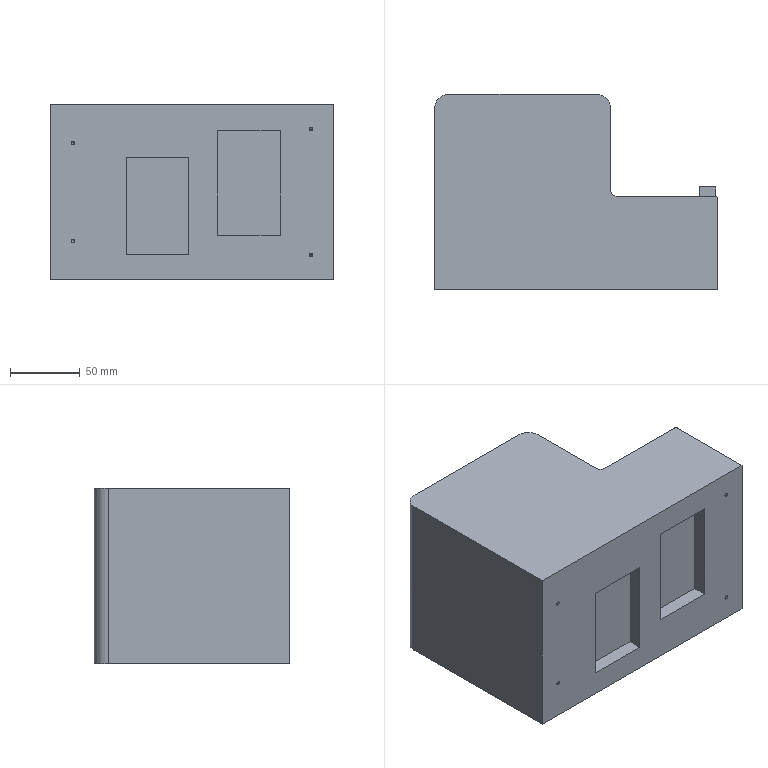Part | 1 solid | 53 faces | box 202.5 x 140 x 126 mm | volume 2802500 mm3 | plane 31 | cylinder 14 | cone 8 | commonest cylinder face diameters 2.5 x8 3 x3 20 x2 8 x1
STEP:
#1=CARTESIAN_POINT('',(16.,11.5,36.25));
#2=VERTEX_POINT('',#1);
#3=CARTESIAN_POINT('',(16.,11.5,33.75));
#4=VERTEX_POINT('',#3);
#5=CARTESIAN_POINT('',(16.,11.5,35.));
#6=DIRECTION('',(0.,-1.,0.));
#7=DIRECTION('',(0.,0.,-1.));
#8=AXIS2_PLACEMENT_3D('',#5,#6,#7);
#9=CIRCLE('',#8,1.25);
#10=EDGE_CURVE('',#2,#4,#9,.T.);
#11=ORIENTED_EDGE('',*,*,#10,.F.);
#12=CARTESIAN_POINT('',(16.,0.,36.25));
#13=VERTEX_POINT('',#12);
#14=CARTESIAN_POINT('',(16.,0.,36.25));
#15=DIRECTION('',(0.,-1.,0.));
#16=VECTOR('',#15,1000.);
#17=LINE('',#14,#16);
#18=EDGE_CURVE('',#2,#13,#17,.T.);
#19=ORIENTED_EDGE('',*,*,#18,.T.);
#20=CARTESIAN_POINT('',(16.,0.,33.75));
#21=VERTEX_POINT('',#20);
#22=CARTESIAN_POINT('',(16.,0.,35.));
#23=DIRECTION('',(0.,-1.,0.));
#24=DIRECTION('',(0.,0.,-1.));
#25=AXIS2_PLACEMENT_3D('',#22,#23,#24);
#26=CIRCLE('',#25,1.25);
#27=EDGE_CURVE('',#13,#21,#26,.T.);
#28=ORIENTED_EDGE('',*,*,#27,.T.);
#29=CARTESIAN_POINT('',(16.,0.,33.75));
#30=DIRECTION('',(0.,-1.,0.));
#31=VECTOR('',#30,1000.);
#32=LINE('',#29,#31);
#33=EDGE_CURVE('',#4,#21,#32,.T.);
#34=ORIENTED_EDGE('',*,*,#33,.F.);
#35=EDGE_LOOP('',(#11,#19,#28,#34));
#36=FACE_OUTER_BOUND('',#35,.T.);
#37=CARTESIAN_POINT('',(16.,0.,35.));
#38=DIRECTION('',(0.,-1.,0.));
#39=DIRECTION('',(0.,0.,-1.));
#40=AXIS2_PLACEMENT_3D('',#37,#38,#39);
#41=CYLINDRICAL_SURFACE('',#40,1.25);
#42=ADVANCED_FACE('',(#36),#41,.F.);
#43=CARTESIAN_POINT('',(16.,12.251,35.));
#44=VERTEX_POINT('',#43);
#45=CARTESIAN_POINT('',(16.,11.5,33.75));
#46=DIRECTION('',(0.,-0.515,-0.8572));
#47=VECTOR('',#46,1000.);
#48=LINE('',#45,#47);
#49=EDGE_CURVE('',#44,#4,#48,.T.);
#50=ORIENTED_EDGE('',*,*,#49,.F.);
#51=CARTESIAN_POINT('',(16.,11.5,36.25));
#52=DIRECTION('',(0.,-0.515,0.8572));
#53=VECTOR('',#52,1000.);
#54=LINE('',#51,#53);
#55=EDGE_CURVE('',#44,#2,#54,.T.);
#56=ORIENTED_EDGE('',*,*,#55,.T.);
#57=ORIENTED_EDGE('',*,*,#10,.T.);
#58=EDGE_LOOP('',(#50,#56,#57));
#59=FACE_OUTER_BOUND('',#58,.T.);
#60=CARTESIAN_POINT('',(16.,11.5,35.));
#61=DIRECTION('',(0.,-1.,0.));
#62=DIRECTION('',(0.,0.,-1.));
#63=AXIS2_PLACEMENT_3D('',#60,#61,#62);
#64=CONICAL_SURFACE('',#63,1.25,1.03);
#65=ADVANCED_FACE('',(#59),#64,.F.);
#66=CARTESIAN_POINT('',(16.,11.5,-33.75));
#67=VERTEX_POINT('',#66);
#68=CARTESIAN_POINT('',(16.,11.5,-36.25));
#69=VERTEX_POINT('',#68);
#70=CARTESIAN_POINT('',(16.,11.5,-35.));
#71=DIRECTION('',(0.,-1.,0.));
#72=DIRECTION('',(0.,0.,-1.));
#73=AXIS2_PLACEMENT_3D('',#70,#71,#72);
#74=CIRCLE('',#73,1.25);
#75=EDGE_CURVE('',#67,#69,#74,.T.);
#76=ORIENTED_EDGE('',*,*,#75,.F.);
#77=CARTESIAN_POINT('',(16.,0.,-33.75));
#78=VERTEX_POINT('',#77);
#79=CARTESIAN_POINT('',(16.,0.,-33.75));
#80=DIRECTION('',(0.,-1.,0.));
#81=VECTOR('',#80,1000.);
#82=LINE('',#79,#81);
#83=EDGE_CURVE('',#67,#78,#82,.T.);
#84=ORIENTED_EDGE('',*,*,#83,.T.);
#85=CARTESIAN_POINT('',(16.,0.,-36.25));
#86=VERTEX_POINT('',#85);
#87=CARTESIAN_POINT('',(16.,0.,-35.));
#88=DIRECTION('',(0.,-1.,0.));
#89=DIRECTION('',(0.,0.,-1.));
#90=AXIS2_PLACEMENT_3D('',#87,#88,#89);
#91=CIRCLE('',#90,1.25);
#92=EDGE_CURVE('',#78,#86,#91,.T.);
#93=ORIENTED_EDGE('',*,*,#92,.T.);
#94=CARTESIAN_POINT('',(16.,0.,-36.25));
#95=DIRECTION('',(0.,-1.,0.));
#96=VECTOR('',#95,1000.);
#97=LINE('',#94,#96);
#98=EDGE_CURVE('',#69,#86,#97,.T.);
#99=ORIENTED_EDGE('',*,*,#98,.F.);
#100=EDGE_LOOP('',(#76,#84,#93,#99));
#101=FACE_OUTER_BOUND('',#100,.T.);
#102=CARTESIAN_POINT('',(16.,0.,-35.));
#103=DIRECTION('',(0.,-1.,0.));
#104=DIRECTION('',(0.,0.,-1.));
#105=AXIS2_PLACEMENT_3D('',#102,#103,#104);
#106=CYLINDRICAL_SURFACE('',#105,1.25);
#107=ADVANCED_FACE('',(#101),#106,.F.);
#108=CARTESIAN_POINT('',(16.,12.251,-35.));
#109=VERTEX_POINT('',#108);
#110=CARTESIAN_POINT('',(16.,11.5,-36.25));
#111=DIRECTION('',(0.,-0.515,-0.8572));
#112=VECTOR('',#111,1000.);
#113=LINE('',#110,#112);
#114=EDGE_CURVE('',#109,#69,#113,.T.);
#115=ORIENTED_EDGE('',*,*,#114,.F.);
#116=CARTESIAN_POINT('',(16.,11.5,-33.75));
#117=DIRECTION('',(0.,-0.515,0.8572));
#118=VECTOR('',#117,1000.);
#119=LINE('',#116,#118);
#120=EDGE_CURVE('',#109,#67,#119,.T.);
#121=ORIENTED_EDGE('',*,*,#120,.T.);
#122=ORIENTED_EDGE('',*,*,#75,.T.);
#123=EDGE_LOOP('',(#115,#121,#122));
#124=FACE_OUTER_BOUND('',#123,.T.);
#125=CARTESIAN_POINT('',(16.,11.5,-35.));
#126=DIRECTION('',(0.,-1.,0.));
#127=DIRECTION('',(0.,0.,-1.));
#128=AXIS2_PLACEMENT_3D('',#125,#126,#127);
#129=CONICAL_SURFACE('',#128,1.25,1.03);
#130=ADVANCED_FACE('',(#124),#129,.F.);
#131=CARTESIAN_POINT('',(186.5,11.5,46.25));
#132=VERTEX_POINT('',#131);
#133=CARTESIAN_POINT('',(186.5,11.5,43.75));
#134=VERTEX_POINT('',#133);
#135=CARTESIAN_POINT('',(186.5,11.5,45.));
#136=DIRECTION('',(0.,-1.,0.));
#137=DIRECTION('',(0.,0.,-1.));
#138=AXIS2_PLACEMENT_3D('',#135,#136,#137);
#139=CIRCLE('',#138,1.25);
#140=EDGE_CURVE('',#132,#134,#139,.T.);
#141=ORIENTED_EDGE('',*,*,#140,.F.);
#142=CARTESIAN_POINT('',(186.5,0.,46.25));
#143=VERTEX_POINT('',#142);
#144=CARTESIAN_POINT('',(186.5,0.,46.25));
#145=DIRECTION('',(0.,-1.,0.));
#146=VECTOR('',#145,1000.);
#147=LINE('',#144,#146);
#148=EDGE_CURVE('',#132,#143,#147,.T.);
#149=ORIENTED_EDGE('',*,*,#148,.T.);
#150=CARTESIAN_POINT('',(186.5,0.,43.75));
#151=VERTEX_POINT('',#150);
#152=CARTESIAN_POINT('',(186.5,0.,45.));
#153=DIRECTION('',(0.,-1.,0.));
#154=DIRECTION('',(0.,0.,-1.));
#155=AXIS2_PLACEMENT_3D('',#152,#153,#154);
#156=CIRCLE('',#155,1.25);
#157=EDGE_CURVE('',#143,#151,#156,.T.);
#158=ORIENTED_EDGE('',*,*,#157,.T.);
#159=CARTESIAN_POINT('',(186.5,0.,43.75));
#160=DIRECTION('',(0.,-1.,0.));
#161=VECTOR('',#160,1000.);
#162=LINE('',#159,#161);
#163=EDGE_CURVE('',#134,#151,#162,.T.);
#164=ORIENTED_EDGE('',*,*,#163,.F.);
#165=EDGE_LOOP('',(#141,#149,#158,#164));
#166=FACE_OUTER_BOUND('',#165,.T.);
#167=CARTESIAN_POINT('',(186.5,0.,45.));
#168=DIRECTION('',(0.,-1.,0.));
#169=DIRECTION('',(0.,0.,-1.));
#170=AXIS2_PLACEMENT_3D('',#167,#168,#169);
#171=CYLINDRICAL_SURFACE('',#170,1.25);
#172=ADVANCED_FACE('',(#166),#171,.F.);
#173=CARTESIAN_POINT('',(186.5,12.251,45.));
#174=VERTEX_POINT('',#173);
#175=CARTESIAN_POINT('',(186.5,11.5,43.75));
#176=DIRECTION('',(0.,-0.515,-0.8572));
#177=VECTOR('',#176,1000.);
#178=LINE('',#175,#177);
#179=EDGE_CURVE('',#174,#134,#178,.T.);
#180=ORIENTED_EDGE('',*,*,#179,.F.);
#181=CARTESIAN_POINT('',(186.5,11.5,46.25));
#182=DIRECTION('',(0.,-0.515,0.8572));
#183=VECTOR('',#182,1000.);
#184=LINE('',#181,#183);
#185=EDGE_CURVE('',#174,#132,#184,.T.);
#186=ORIENTED_EDGE('',*,*,#185,.T.);
#187=ORIENTED_EDGE('',*,*,#140,.T.);
#188=EDGE_LOOP('',(#180,#186,#187));
#189=FACE_OUTER_BOUND('',#188,.T.);
#190=CARTESIAN_POINT('',(186.5,11.5,45.));
#191=DIRECTION('',(0.,-1.,0.));
#192=DIRECTION('',(0.,0.,-1.));
#193=AXIS2_PLACEMENT_3D('',#190,#191,#192);
#194=CONICAL_SURFACE('',#193,1.25,1.03);
#195=ADVANCED_FACE('',(#189),#194,.F.);
#196=CARTESIAN_POINT('',(186.5,11.5,-43.75));
#197=VERTEX_POINT('',#196);
#198=CARTESIAN_POINT('',(186.5,11.5,-46.25));
#199=VERTEX_POINT('',#198);
#200=CARTESIAN_POINT('',(186.5,11.5,-45.));
#201=DIRECTION('',(0.,-1.,0.));
#202=DIRECTION('',(0.,0.,-1.));
#203=AXIS2_PLACEMENT_3D('',#200,#201,#202);
#204=CIRCLE('',#203,1.25);
#205=EDGE_CURVE('',#197,#199,#204,.T.);
#206=ORIENTED_EDGE('',*,*,#205,.F.);
#207=CARTESIAN_POINT('',(186.5,0.,-43.75));
#208=VERTEX_POINT('',#207);
#209=CARTESIAN_POINT('',(186.5,0.,-43.75));
#210=DIRECTION('',(0.,-1.,0.));
#211=VECTOR('',#210,1000.);
#212=LINE('',#209,#211);
#213=EDGE_CURVE('',#197,#208,#212,.T.);
#214=ORIENTED_EDGE('',*,*,#213,.T.);
#215=CARTESIAN_POINT('',(186.5,0.,-46.25));
#216=VERTEX_POINT('',#215);
#217=CARTESIAN_POINT('',(186.5,0.,-45.));
#218=DIRECTION('',(0.,-1.,0.));
#219=DIRECTION('',(0.,0.,-1.));
#220=AXIS2_PLACEMENT_3D('',#217,#218,#219);
#221=CIRCLE('',#220,1.25);
#222=EDGE_CURVE('',#208,#216,#221,.T.);
#223=ORIENTED_EDGE('',*,*,#222,.T.);
#224=CARTESIAN_POINT('',(186.5,0.,-46.25));
#225=DIRECTION('',(0.,-1.,0.));
#226=VECTOR('',#225,1000.);
#227=LINE('',#224,#226);
#228=EDGE_CURVE('',#199,#216,#227,.T.);
#229=ORIENTED_EDGE('',*,*,#228,.F.);
#230=EDGE_LOOP('',(#206,#214,#223,#229));
#231=FACE_OUTER_BOUND('',#230,.T.);
#232=CARTESIAN_POINT('',(186.5,0.,-45.));
#233=DIRECTION('',(0.,-1.,0.));
#234=DIRECTION('',(0.,0.,-1.));
#235=AXIS2_PLACEMENT_3D('',#232,#233,#234);
#236=CYLINDRICAL_SURFACE('',#235,1.25);
#237=ADVANCED_FACE('',(#231),#236,.F.);
#238=CARTESIAN_POINT('',(186.5,12.251,-45.));
#239=VERTEX_POINT('',#238);
#240=CARTESIAN_POINT('',(186.5,11.5,-46.25));
#241=DIRECTION('',(0.,-0.515,-0.8572));
#242=VECTOR('',#241,1000.);
#243=LINE('',#240,#242);
#244=EDGE_CURVE('',#239,#199,#243,.T.);
#245=ORIENTED_EDGE('',*,*,#244,.F.);
#246=CARTESIAN_POINT('',(186.5,11.5,-43.75));
#247=DIRECTION('',(0.,-0.515,0.8572));
#248=VECTOR('',#247,1000.);
#249=LINE('',#246,#248);
#250=EDGE_CURVE('',#239,#197,#249,.T.);
#251=ORIENTED_EDGE('',*,*,#250,.T.);
#252=ORIENTED_EDGE('',*,*,#205,.T.);
#253=EDGE_LOOP('',(#245,#251,#252));
#254=FACE_OUTER_BOUND('',#253,.T.);
#255=CARTESIAN_POINT('',(186.5,11.5,-45.));
#256=DIRECTION('',(0.,-1.,0.));
#257=DIRECTION('',(0.,0.,-1.));
#258=AXIS2_PLACEMENT_3D('',#255,#256,#257);
#259=CONICAL_SURFACE('',#258,1.25,1.03);
#260=ADVANCED_FACE('',(#254),#259,.F.);
#261=CARTESIAN_POINT('',(195.72,57.,-0.5));
#262=VERTEX_POINT('',#261);
#263=CARTESIAN_POINT('',(192.72,57.,-0.5));
#264=VERTEX_POINT('',#263);
#265=CARTESIAN_POINT('',(194.22,57.,-0.5));
#266=DIRECTION('',(0.,1.,0.));
#267=DIRECTION('',(-1.,0.,0.));
#268=AXIS2_PLACEMENT_3D('',#265,#266,#267);
#269=CIRCLE('',#268,1.5);
#270=EDGE_CURVE('',#262,#264,#269,.T.);
#271=ORIENTED_EDGE('',*,*,#270,.F.);
#272=CARTESIAN_POINT('',(195.72,67.,-0.5));
#273=VERTEX_POINT('',#272);
#274=CARTESIAN_POINT('',(195.72,57.,-0.5));
#275=DIRECTION('',(0.,1.,0.));
#276=VECTOR('',#275,1000.);
#277=LINE('',#274,#276);
#278=EDGE_CURVE('',#262,#273,#277,.T.);
#279=ORIENTED_EDGE('',*,*,#278,.T.);
#280=CARTESIAN_POINT('',(192.72,67.,-0.5));
#281=VERTEX_POINT('',#280);
#282=CARTESIAN_POINT('',(194.22,67.,-0.5));
#283=DIRECTION('',(0.,1.,0.));
#284=DIRECTION('',(-1.,0.,0.));
#285=AXIS2_PLACEMENT_3D('',#282,#283,#284);
#286=CIRCLE('',#285,1.5);
#287=EDGE_CURVE('',#273,#281,#286,.T.);
#288=ORIENTED_EDGE('',*,*,#287,.T.);
#289=CARTESIAN_POINT('',(192.72,57.,-0.5));
#290=DIRECTION('',(0.,1.,0.));
#291=VECTOR('',#290,1000.);
#292=LINE('',#289,#291);
#293=EDGE_CURVE('',#264,#281,#292,.T.);
#294=ORIENTED_EDGE('',*,*,#293,.F.);
#295=EDGE_LOOP('',(#271,#279,#288,#294));
#296=FACE_OUTER_BOUND('',#295,.T.);
#297=CARTESIAN_POINT('',(194.22,57.,-0.5));
#298=DIRECTION('',(0.,1.,0.));
#299=DIRECTION('',(-1.,0.,0.));
#300=AXIS2_PLACEMENT_3D('',#297,#298,#299);
#301=CYLINDRICAL_SURFACE('',#300,1.5);
#302=ADVANCED_FACE('',(#296),#301,.F.);
#303=CARTESIAN_POINT('',(194.22,67.,-0.5));
#304=DIRECTION('',(0.,1.,0.));
#305=DIRECTION('',(-1.,0.,0.));
#306=AXIS2_PLACEMENT_3D('',#303,#304,#305);
#307=CIRCLE('',#306,1.5);
#308=EDGE_CURVE('',#281,#273,#307,.T.);
#309=ORIENTED_EDGE('',*,*,#308,.F.);
#310=ORIENTED_EDGE('',*,*,#287,.F.);
#311=EDGE_LOOP('',(#309,#310));
#312=FACE_BOUND('',#311,.T.);
#313=CARTESIAN_POINT('',(201.,67.,-63.));
#314=VERTEX_POINT('',#313);
#315=CARTESIAN_POINT('',(130.,67.,-63.));
#316=VERTEX_POINT('',#315);
#317=CARTESIAN_POINT('',(202.5,67.,-63.));
#318=DIRECTION('',(-1.,0.,0.));
#319=VECTOR('',#318,1000.);
#320=LINE('',#317,#319);
#321=EDGE_CURVE('',#314,#316,#320,.T.);
#322=ORIENTED_EDGE('',*,*,#321,.T.);
#323=CARTESIAN_POINT('',(130.,67.,63.));
#324=VERTEX_POINT('',#323);
#325=CARTESIAN_POINT('',(130.,67.,63.));
#326=DIRECTION('',(0.,0.,1.));
#327=VECTOR('',#326,1000.);
#328=LINE('',#325,#327);
#329=EDGE_CURVE('',#316,#324,#328,.T.);
#330=ORIENTED_EDGE('',*,*,#329,.T.);
#331=CARTESIAN_POINT('',(201.,67.,63.));
#332=VERTEX_POINT('',#331);
#333=CARTESIAN_POINT('',(202.5,67.,63.));
#334=DIRECTION('',(-1.,0.,0.));
#335=VECTOR('',#334,1000.);
#336=LINE('',#333,#335);
#337=EDGE_CURVE('',#332,#324,#336,.T.);
#338=ORIENTED_EDGE('',*,*,#337,.F.);
#339=CARTESIAN_POINT('',(201.,67.,53.5));
#340=VERTEX_POINT('',#339);
#341=CARTESIAN_POINT('',(201.,67.,63.));
#342=DIRECTION('',(0.,0.,-1.));
#343=VECTOR('',#342,1000.);
#344=LINE('',#341,#343);
#345=EDGE_CURVE('',#332,#340,#344,.T.);
#346=ORIENTED_EDGE('',*,*,#345,.T.);
#347=CARTESIAN_POINT('',(190.,67.,53.5));
#348=VERTEX_POINT('',#347);
#349=CARTESIAN_POINT('',(190.,67.,53.5));
#350=DIRECTION('',(1.,0.,0.));
#351=VECTOR('',#350,1000.);
#352=LINE('',#349,#351);
#353=EDGE_CURVE('',#348,#340,#352,.T.);
#354=ORIENTED_EDGE('',*,*,#353,.F.);
#355=CARTESIAN_POINT('',(190.,67.,22.5));
#356=VERTEX_POINT('',#355);
#357=CARTESIAN_POINT('',(190.,67.,22.5));
#358=DIRECTION('',(0.,0.,1.));
#359=VECTOR('',#358,1000.);
#360=LINE('',#357,#359);
#361=EDGE_CURVE('',#356,#348,#360,.T.);
#362=ORIENTED_EDGE('',*,*,#361,.F.);
#363=CARTESIAN_POINT('',(201.,67.,22.5));
#364=VERTEX_POINT('',#363);
#365=CARTESIAN_POINT('',(190.,67.,22.5));
#366=DIRECTION('',(-1.,0.,0.));
#367=VECTOR('',#366,1000.);
#368=LINE('',#365,#367);
#369=EDGE_CURVE('',#364,#356,#368,.T.);
#370=ORIENTED_EDGE('',*,*,#369,.F.);
#371=CARTESIAN_POINT('',(201.,67.,-15.5));
#372=VERTEX_POINT('',#371);
#373=CARTESIAN_POINT('',(201.,67.,63.));
#374=DIRECTION('',(0.,0.,-1.));
#375=VECTOR('',#374,1000.);
#376=LINE('',#373,#375);
#377=EDGE_CURVE('',#364,#372,#376,.T.);
#378=ORIENTED_EDGE('',*,*,#377,.T.);
#379=CARTESIAN_POINT('',(190.,67.,-15.5));
#380=VERTEX_POINT('',#379);
#381=CARTESIAN_POINT('',(190.,67.,-15.5));
#382=DIRECTION('',(1.,0.,0.));
#383=VECTOR('',#382,1000.);
#384=LINE('',#381,#383);
#385=EDGE_CURVE('',#380,#372,#384,.T.);
#386=ORIENTED_EDGE('',*,*,#385,.F.);
#387=CARTESIAN_POINT('',(190.,67.,-46.5));
#388=VERTEX_POINT('',#387);
#389=CARTESIAN_POINT('',(190.,67.,-46.5));
#390=DIRECTION('',(0.,0.,1.));
#391=VECTOR('',#390,1000.);
#392=LINE('',#389,#391);
#393=EDGE_CURVE('',#388,#380,#392,.T.);
#394=ORIENTED_EDGE('',*,*,#393,.F.);
#395=CARTESIAN_POINT('',(201.,67.,-46.5));
#396=VERTEX_POINT('',#395);
#397=CARTESIAN_POINT('',(190.,67.,-46.5));
#398=DIRECTION('',(-1.,0.,0.));
#399=VECTOR('',#398,1000.);
#400=LINE('',#397,#399);
#401=EDGE_CURVE('',#396,#388,#400,.T.);
#402=ORIENTED_EDGE('',*,*,#401,.F.);
#403=CARTESIAN_POINT('',(201.,67.,63.));
#404=DIRECTION('',(0.,0.,-1.));
#405=VECTOR('',#404,1000.);
#406=LINE('',#403,#405);
#407=EDGE_CURVE('',#396,#314,#406,.T.);
#408=ORIENTED_EDGE('',*,*,#407,.T.);
#409=EDGE_LOOP('',(#322,#330,#338,#346,#354,#362,#370,#378,#386,#394,#402,#408));
#410=FACE_OUTER_BOUND('',#409,.T.);
#411=CARTESIAN_POINT('',(202.5,67.,63.));
#412=DIRECTION('',(0.,-1.,0.));
#413=DIRECTION('',(1.,0.,0.));
#414=AXIS2_PLACEMENT_3D('',#411,#412,#413);
#415=PLANE('',#414);
#416=ADVANCED_FACE('',(#312,#410),#415,.F.);
#417=CARTESIAN_POINT('',(116.,140.,63.));
#418=VERTEX_POINT('',#417);
#419=CARTESIAN_POINT('',(10.,140.,63.));
#420=VERTEX_POINT('',#419);
#421=CARTESIAN_POINT('',(126.,140.,63.));
#422=DIRECTION('',(-1.,0.,0.));
#423=VECTOR('',#422,1000.);
#424=LINE('',#421,#423);
#425=EDGE_CURVE('',#418,#420,#424,.T.);
#426=ORIENTED_EDGE('',*,*,#425,.F.);
#427=CARTESIAN_POINT('',(116.,140.,-63.));
#428=VERTEX_POINT('',#427);
#429=CARTESIAN_POINT('',(116.,140.,63.));
#430=DIRECTION('',(0.,0.,-1.));
#431=VECTOR('',#430,1000.);
#432=LINE('',#429,#431);
#433=EDGE_CURVE('',#418,#428,#432,.T.);
#434=ORIENTED_EDGE('',*,*,#433,.T.);
#435=CARTESIAN_POINT('',(10.,140.,-63.));
#436=VERTEX_POINT('',#435);
#437=CARTESIAN_POINT('',(126.,140.,-63.));
#438=DIRECTION('',(-1.,0.,0.));
#439=VECTOR('',#438,1000.);
#440=LINE('',#437,#439);
#441=EDGE_CURVE('',#428,#436,#440,.T.);
#442=ORIENTED_EDGE('',*,*,#441,.T.);
#443=CARTESIAN_POINT('',(10.,140.,63.));
#444=DIRECTION('',(0.,0.,1.));
#445=VECTOR('',#444,1000.);
#446=LINE('',#443,#445);
#447=EDGE_CURVE('',#436,#420,#446,.T.);
#448=ORIENTED_EDGE('',*,*,#447,.T.);
#449=EDGE_LOOP('',(#426,#434,#442,#448));
#450=FACE_OUTER_BOUND('',#449,.T.);
#451=CARTESIAN_POINT('',(126.,140.,63.));
#452=DIRECTION('',(0.,-1.,0.));
#453=DIRECTION('',(1.,0.,0.));
#454=AXIS2_PLACEMENT_3D('',#451,#452,#453);
#455=PLANE('',#454);
#456=ADVANCED_FACE('',(#450),#455,.F.);
#457=CARTESIAN_POINT('',(0.,130.,63.));
#458=VERTEX_POINT('',#457);
#459=CARTESIAN_POINT('',(0.,0.,63.));
#460=VERTEX_POINT('',#459);
#461=CARTESIAN_POINT('',(0.,140.,63.));
#462=DIRECTION('',(0.,-1.,0.));
#463=VECTOR('',#462,1000.);
#464=LINE('',#461,#463);
#465=EDGE_CURVE('',#458,#460,#464,.T.);
#466=ORIENTED_EDGE('',*,*,#465,.F.);
#467=CARTESIAN_POINT('',(0.,130.,-63.));
#468=VERTEX_POINT('',#467);
#469=CARTESIAN_POINT('',(0.,130.,63.));
#470=DIRECTION('',(0.,0.,-1.));
#471=VECTOR('',#470,1000.);
#472=LINE('',#469,#471);
#473=EDGE_CURVE('',#458,#468,#472,.T.);
#474=ORIENTED_EDGE('',*,*,#473,.T.);
#475=CARTESIAN_POINT('',(0.,0.,-63.));
#476=VERTEX_POINT('',#475);
#477=CARTESIAN_POINT('',(0.,140.,-63.));
#478=DIRECTION('',(0.,-1.,0.));
#479=VECTOR('',#478,1000.);
#480=LINE('',#477,#479);
#481=EDGE_CURVE('',#468,#476,#480,.T.);
#482=ORIENTED_EDGE('',*,*,#481,.T.);
#483=CARTESIAN_POINT('',(0.,0.,63.));
#484=DIRECTION('',(0.,0.,-1.));
#485=VECTOR('',#484,1000.);
#486=LINE('',#483,#485);
#487=EDGE_CURVE('',#460,#476,#486,.T.);
#488=ORIENTED_EDGE('',*,*,#487,.F.);
#489=EDGE_LOOP('',(#466,#474,#482,#488));
#490=FACE_OUTER_BOUND('',#489,.T.);
#491=CARTESIAN_POINT('',(0.,140.,63.));
#492=DIRECTION('',(1.,0.,0.));
#493=DIRECTION('',(0.,1.,0.));
#494=AXIS2_PLACEMENT_3D('',#491,#492,#493);
#495=PLANE('',#494);
#496=ADVANCED_FACE('',(#490),#495,.F.);
#497=CARTESIAN_POINT('',(164.5,0.,44.));
#498=VERTEX_POINT('',#497);
#499=CARTESIAN_POINT('',(119.5,0.,44.));
#500=VERTEX_POINT('',#499);
#501=CARTESIAN_POINT('',(119.5,0.,44.));
#502=DIRECTION('',(-1.,0.,0.));
#503=VECTOR('',#502,1000.);
#504=LINE('',#501,#503);
#505=EDGE_CURVE('',#498,#500,#504,.T.);
#506=ORIENTED_EDGE('',*,*,#505,.F.);
#507=CARTESIAN_POINT('',(164.5,0.,-31.));
#508=VERTEX_POINT('',#507);
#509=CARTESIAN_POINT('',(164.5,0.,44.));
#510=DIRECTION('',(0.,0.,1.));
#511=VECTOR('',#510,1000.);
#512=LINE('',#509,#511);
#513=EDGE_CURVE('',#508,#498,#512,.T.);
#514=ORIENTED_EDGE('',*,*,#513,.F.);
#515=CARTESIAN_POINT('',(119.5,0.,-31.));
#516=VERTEX_POINT('',#515);
#517=CARTESIAN_POINT('',(119.5,0.,-31.));
#518=DIRECTION('',(1.,0.,0.));
#519=VECTOR('',#518,1000.);
#520=LINE('',#517,#519);
#521=EDGE_CURVE('',#516,#508,#520,.T.);
#522=ORIENTED_EDGE('',*,*,#521,.F.);
#523=CARTESIAN_POINT('',(119.5,0.,44.));
#524=DIRECTION('',(0.,0.,-1.));
#525=VECTOR('',#524,1000.);
#526=LINE('',#523,#525);
#527=EDGE_CURVE('',#500,#516,#526,.T.);
#528=ORIENTED_EDGE('',*,*,#527,.F.);
#529=EDGE_LOOP('',(#506,#514,#522,#528));
#530=FACE_BOUND('',#529,.T.);
#531=CARTESIAN_POINT('',(99.,0.,25.));
#532=VERTEX_POINT('',#531);
#533=CARTESIAN_POINT('',(54.,0.,25.));
#534=VERTEX_POINT('',#533);
#535=CARTESIAN_POINT('',(54.,0.,25.));
#536=DIRECTION('',(-1.,0.,0.));
#537=VECTOR('',#536,1000.);
#538=LINE('',#535,#537);
#539=EDGE_CURVE('',#532,#534,#538,.T.);
#540=ORIENTED_EDGE('',*,*,#539,.F.);
#541=CARTESIAN_POINT('',(99.,0.,-45.));
#542=VERTEX_POINT('',#541);
#543=CARTESIAN_POINT('',(99.,0.,25.));
#544=DIRECTION('',(0.,0.,1.));
#545=VECTOR('',#544,1000.);
#546=LINE('',#543,#545);
#547=EDGE_CURVE('',#542,#532,#546,.T.);
#548=ORIENTED_EDGE('',*,*,#547,.F.);
#549=CARTESIAN_POINT('',(54.,0.,-45.));
#550=VERTEX_POINT('',#549);
#551=CARTESIAN_POINT('',(54.,0.,-45.));
#552=DIRECTION('',(1.,0.,0.));
#553=VECTOR('',#552,1000.);
#554=LINE('',#551,#553);
#555=EDGE_CURVE('',#550,#542,#554,.T.);
#556=ORIENTED_EDGE('',*,*,#555,.F.);
#557=CARTESIAN_POINT('',(54.,0.,25.));
#558=DIRECTION('',(0.,0.,-1.));
#559=VECTOR('',#558,1000.);
#560=LINE('',#557,#559);
#561=EDGE_CURVE('',#534,#550,#560,.T.);
#562=ORIENTED_EDGE('',*,*,#561,.F.);
#563=EDGE_LOOP('',(#540,#548,#556,#562));
#564=FACE_BOUND('',#563,.T.);
#565=CARTESIAN_POINT('',(16.,0.,35.));
#566=DIRECTION('',(0.,-1.,0.));
#567=DIRECTION('',(0.,0.,-1.));
#568=AXIS2_PLACEMENT_3D('',#565,#566,#567);
#569=CIRCLE('',#568,1.25);
#570=EDGE_CURVE('',#21,#13,#569,.T.);
#571=ORIENTED_EDGE('',*,*,#570,.F.);
#572=ORIENTED_EDGE('',*,*,#27,.F.);
#573=EDGE_LOOP('',(#571,#572));
#574=FACE_BOUND('',#573,.T.);
#575=CARTESIAN_POINT('',(16.,0.,-35.));
#576=DIRECTION('',(0.,-1.,0.));
#577=DIRECTION('',(0.,0.,-1.));
#578=AXIS2_PLACEMENT_3D('',#575,#576,#577);
#579=CIRCLE('',#578,1.25);
#580=EDGE_CURVE('',#86,#78,#579,.T.);
#581=ORIENTED_EDGE('',*,*,#580,.F.);
#582=ORIENTED_EDGE('',*,*,#92,.F.);
#583=EDGE_LOOP('',(#581,#582));
#584=FACE_BOUND('',#583,.T.);
#585=CARTESIAN_POINT('',(186.5,0.,45.));
#586=DIRECTION('',(0.,-1.,0.));
#587=DIRECTION('',(0.,0.,-1.));
#588=AXIS2_PLACEMENT_3D('',#585,#586,#587);
#589=CIRCLE('',#588,1.25);
#590=EDGE_CURVE('',#151,#143,#589,.T.);
#591=ORIENTED_EDGE('',*,*,#590,.F.);
#592=ORIENTED_EDGE('',*,*,#157,.F.);
#593=EDGE_LOOP('',(#591,#592));
#594=FACE_BOUND('',#593,.T.);
#595=CARTESIAN_POINT('',(186.5,0.,-45.));
#596=DIRECTION('',(0.,-1.,0.));
#597=DIRECTION('',(0.,0.,-1.));
#598=AXIS2_PLACEMENT_3D('',#595,#596,#597);
#599=CIRCLE('',#598,1.25);
#600=EDGE_CURVE('',#216,#208,#599,.T.);
#601=ORIENTED_EDGE('',*,*,#600,.F.);
#602=ORIENTED_EDGE('',*,*,#222,.F.);
#603=EDGE_LOOP('',(#601,#602));
#604=FACE_BOUND('',#603,.T.);
#605=CARTESIAN_POINT('',(202.5,0.,-63.));
#606=VERTEX_POINT('',#605);
#607=CARTESIAN_POINT('',(0.,0.,-63.));
#608=DIRECTION('',(1.,0.,0.));
#609=VECTOR('',#608,1000.);
#610=LINE('',#607,#609);
#611=EDGE_CURVE('',#476,#606,#610,.T.);
#612=ORIENTED_EDGE('',*,*,#611,.T.);
#613=CARTESIAN_POINT('',(202.5,0.,63.));
#614=VERTEX_POINT('',#613);
#615=CARTESIAN_POINT('',(202.5,0.,63.));
#616=DIRECTION('',(0.,0.,-1.));
#617=VECTOR('',#616,1000.);
#618=LINE('',#615,#617);
#619=EDGE_CURVE('',#614,#606,#618,.T.);
#620=ORIENTED_EDGE('',*,*,#619,.F.);
#621=CARTESIAN_POINT('',(0.,0.,63.));
#622=DIRECTION('',(1.,0.,0.));
#623=VECTOR('',#622,1000.);
#624=LINE('',#621,#623);
#625=EDGE_CURVE('',#460,#614,#624,.T.);
#626=ORIENTED_EDGE('',*,*,#625,.F.);
#627=ORIENTED_EDGE('',*,*,#487,.T.);
#628=EDGE_LOOP('',(#612,#620,#626,#627));
#629=FACE_OUTER_BOUND('',#628,.T.);
#630=CARTESIAN_POINT('',(0.,0.,63.));
#631=DIRECTION('',(0.,1.,0.));
#632=DIRECTION('',(0.,0.,1.));
#633=AXIS2_PLACEMENT_3D('',#630,#631,#632);
#634=PLANE('',#633);
#635=ADVANCED_FACE('',(#530,#564,#574,#584,#594,#604,#629),#634,.F.);
#636=CARTESIAN_POINT('',(202.5,65.5,-63.));
#637=VERTEX_POINT('',#636);
#638=CARTESIAN_POINT('',(202.5,0.,-63.));
#639=DIRECTION('',(0.,1.,0.));
#640=VECTOR('',#639,1000.);
#641=LINE('',#638,#640);
#642=EDGE_CURVE('',#606,#637,#641,.T.);
#643=ORIENTED_EDGE('',*,*,#642,.T.);
#644=CARTESIAN_POINT('',(202.5,65.5,63.));
#645=VERTEX_POINT('',#644);
#646=CARTESIAN_POINT('',(202.5,65.5,63.));
#647=DIRECTION('',(0.,0.,1.));
#648=VECTOR('',#647,1000.);
#649=LINE('',#646,#648);
#650=EDGE_CURVE('',#637,#645,#649,.T.);
#651=ORIENTED_EDGE('',*,*,#650,.T.);
#652=CARTESIAN_POINT('',(202.5,0.,63.));
#653=DIRECTION('',(0.,1.,0.));
#654=VECTOR('',#653,1000.);
#655=LINE('',#652,#654);
#656=EDGE_CURVE('',#614,#645,#655,.T.);
#657=ORIENTED_EDGE('',*,*,#656,.F.);
#658=ORIENTED_EDGE('',*,*,#619,.T.);
#659=EDGE_LOOP('',(#643,#651,#657,#658));
#660=FACE_OUTER_BOUND('',#659,.T.);
#661=CARTESIAN_POINT('',(202.5,0.,63.));
#662=DIRECTION('',(-1.,0.,0.));
#663=DIRECTION('',(0.,0.,1.));
#664=AXIS2_PLACEMENT_3D('',#661,#662,#663);
#665=PLANE('',#664);
#666=ADVANCED_FACE('',(#660),#665,.F.);
#667=CARTESIAN_POINT('',(126.,71.,63.));
#668=VERTEX_POINT('',#667);
#669=CARTESIAN_POINT('',(126.,130.,63.));
#670=VERTEX_POINT('',#669);
#671=CARTESIAN_POINT('',(126.,67.,63.));
#672=DIRECTION('',(0.,1.,0.));
#673=VECTOR('',#672,1000.);
#674=LINE('',#671,#673);
#675=EDGE_CURVE('',#668,#670,#674,.T.);
#676=ORIENTED_EDGE('',*,*,#675,.F.);
#677=CARTESIAN_POINT('',(126.,71.,-63.));
#678=VERTEX_POINT('',#677);
#679=CARTESIAN_POINT('',(126.,71.,-63.));
#680=DIRECTION('',(0.,0.,-1.));
#681=VECTOR('',#680,1000.);
#682=LINE('',#679,#681);
#683=EDGE_CURVE('',#668,#678,#682,.T.);
#684=ORIENTED_EDGE('',*,*,#683,.T.);
#685=CARTESIAN_POINT('',(126.,130.,-63.));
#686=VERTEX_POINT('',#685);
#687=CARTESIAN_POINT('',(126.,67.,-63.));
#688=DIRECTION('',(0.,1.,0.));
#689=VECTOR('',#688,1000.);
#690=LINE('',#687,#689);
#691=EDGE_CURVE('',#678,#686,#690,.T.);
#692=ORIENTED_EDGE('',*,*,#691,.T.);
#693=CARTESIAN_POINT('',(126.,130.,63.));
#694=DIRECTION('',(0.,0.,1.));
#695=VECTOR('',#694,1000.);
#696=LINE('',#693,#695);
#697=EDGE_CURVE('',#686,#670,#696,.T.);
#698=ORIENTED_EDGE('',*,*,#697,.T.);
#699=EDGE_LOOP('',(#676,#684,#692,#698));
#700=FACE_OUTER_BOUND('',#699,.T.);
#701=CARTESIAN_POINT('',(126.,67.,63.));
#702=DIRECTION('',(-1.,0.,0.));
#703=DIRECTION('',(0.,0.,1.));
#704=AXIS2_PLACEMENT_3D('',#701,#702,#703);
#705=PLANE('',#704);
#706=ADVANCED_FACE('',(#700),#705,.F.);
#707=ORIENTED_EDGE('',*,*,#656,.T.);
#708=CARTESIAN_POINT('',(201.,65.5,63.));
#709=DIRECTION('',(0.,0.,1.));
#710=DIRECTION('',(1.,0.,0.));
#711=AXIS2_PLACEMENT_3D('',#708,#709,#710);
#712=CIRCLE('',#711,1.5);
#713=EDGE_CURVE('',#645,#332,#712,.T.);
#714=ORIENTED_EDGE('',*,*,#713,.T.);
#715=ORIENTED_EDGE('',*,*,#337,.T.);
#716=CARTESIAN_POINT('',(130.,71.,63.));
#717=DIRECTION('',(0.,0.,-1.));
#718=DIRECTION('',(1.,0.,0.));
#719=AXIS2_PLACEMENT_3D('',#716,#717,#718);
#720=CIRCLE('',#719,4.);
#721=EDGE_CURVE('',#324,#668,#720,.T.);
#722=ORIENTED_EDGE('',*,*,#721,.T.);
#723=ORIENTED_EDGE('',*,*,#675,.T.);
#724=CARTESIAN_POINT('',(116.,130.,63.));
#725=DIRECTION('',(0.,0.,1.));
#726=DIRECTION('',(1.,0.,0.));
#727=AXIS2_PLACEMENT_3D('',#724,#725,#726);
#728=CIRCLE('',#727,10.);
#729=EDGE_CURVE('',#670,#418,#728,.T.);
#730=ORIENTED_EDGE('',*,*,#729,.T.);
#731=ORIENTED_EDGE('',*,*,#425,.T.);
#732=CARTESIAN_POINT('',(10.,130.,63.));
#733=DIRECTION('',(0.,0.,1.));
#734=DIRECTION('',(1.,0.,0.));
#735=AXIS2_PLACEMENT_3D('',#732,#733,#734);
#736=CIRCLE('',#735,10.);
#737=EDGE_CURVE('',#420,#458,#736,.T.);
#738=ORIENTED_EDGE('',*,*,#737,.T.);
#739=ORIENTED_EDGE('',*,*,#465,.T.);
#740=ORIENTED_EDGE('',*,*,#625,.T.);
#741=EDGE_LOOP('',(#707,#714,#715,#722,#723,#730,#731,#738,#739,#740));
#742=FACE_OUTER_BOUND('',#741,.T.);
#743=CARTESIAN_POINT('',(0.,0.,63.));
#744=DIRECTION('',(0.,0.,1.));
#745=DIRECTION('',(1.,0.,0.));
#746=AXIS2_PLACEMENT_3D('',#743,#744,#745);
#747=PLANE('',#746);
#748=ADVANCED_FACE('',(#742),#747,.T.);
#749=ORIENTED_EDGE('',*,*,#321,.F.);
#750=CARTESIAN_POINT('',(201.,65.5,-63.));
#751=DIRECTION('',(0.,0.,-1.));
#752=DIRECTION('',(1.,0.,0.));
#753=AXIS2_PLACEMENT_3D('',#750,#751,#752);
#754=CIRCLE('',#753,1.5);
#755=EDGE_CURVE('',#314,#637,#754,.T.);
#756=ORIENTED_EDGE('',*,*,#755,.T.);
#757=ORIENTED_EDGE('',*,*,#642,.F.);
#758=ORIENTED_EDGE('',*,*,#611,.F.);
#759=ORIENTED_EDGE('',*,*,#481,.F.);
#760=CARTESIAN_POINT('',(10.,130.,-63.));
#761=DIRECTION('',(0.,0.,-1.));
#762=DIRECTION('',(1.,0.,0.));
#763=AXIS2_PLACEMENT_3D('',#760,#761,#762);
#764=CIRCLE('',#763,10.);
#765=EDGE_CURVE('',#468,#436,#764,.T.);
#766=ORIENTED_EDGE('',*,*,#765,.T.);
#767=ORIENTED_EDGE('',*,*,#441,.F.);
#768=CARTESIAN_POINT('',(116.,130.,-63.));
#769=DIRECTION('',(0.,0.,-1.));
#770=DIRECTION('',(1.,0.,0.));
#771=AXIS2_PLACEMENT_3D('',#768,#769,#770);
#772=CIRCLE('',#771,10.);
#773=EDGE_CURVE('',#428,#686,#772,.T.);
#774=ORIENTED_EDGE('',*,*,#773,.T.);
#775=ORIENTED_EDGE('',*,*,#691,.F.);
#776=CARTESIAN_POINT('',(130.,71.,-63.));
#777=DIRECTION('',(0.,0.,1.));
#778=DIRECTION('',(1.,0.,0.));
#779=AXIS2_PLACEMENT_3D('',#776,#777,#778);
#780=CIRCLE('',#779,4.);
#781=EDGE_CURVE('',#678,#316,#780,.T.);
#782=ORIENTED_EDGE('',*,*,#781,.T.);
#783=EDGE_LOOP('',(#749,#756,#757,#758,#759,#766,#767,#774,#775,#782));
#784=FACE_OUTER_BOUND('',#783,.T.);
#785=CARTESIAN_POINT('',(0.,0.,-63.));
#786=DIRECTION('',(0.,0.,1.));
#787=DIRECTION('',(1.,0.,0.));
#788=AXIS2_PLACEMENT_3D('',#785,#786,#787);
#789=PLANE('',#788);
#790=ADVANCED_FACE('',(#784),#789,.F.);
#791=ORIENTED_EDGE('',*,*,#729,.F.);
#792=ORIENTED_EDGE('',*,*,#697,.F.);
#793=ORIENTED_EDGE('',*,*,#773,.F.);
#794=ORIENTED_EDGE('',*,*,#433,.F.);
#795=EDGE_LOOP('',(#791,#792,#793,#794));
#796=FACE_OUTER_BOUND('',#795,.T.);
#797=CARTESIAN_POINT('',(116.,130.,63.));
#798=DIRECTION('',(0.,0.,-1.));
#799=DIRECTION('',(-1.,0.,0.));
#800=AXIS2_PLACEMENT_3D('',#797,#798,#799);
#801=CYLINDRICAL_SURFACE('',#800,10.);
#802=ADVANCED_FACE('',(#796),#801,.T.);
#803=ORIENTED_EDGE('',*,*,#737,.F.);
#804=ORIENTED_EDGE('',*,*,#447,.F.);
#805=ORIENTED_EDGE('',*,*,#765,.F.);
#806=ORIENTED_EDGE('',*,*,#473,.F.);
#807=EDGE_LOOP('',(#803,#804,#805,#806));
#808=FACE_OUTER_BOUND('',#807,.T.);
#809=CARTESIAN_POINT('',(10.,130.,63.));
#810=DIRECTION('',(0.,0.,-1.));
#811=DIRECTION('',(-1.,0.,0.));
#812=AXIS2_PLACEMENT_3D('',#809,#810,#811);
#813=CYLINDRICAL_SURFACE('',#812,10.);
#814=ADVANCED_FACE('',(#808),#813,.T.);
#815=ORIENTED_EDGE('',*,*,#713,.F.);
#816=ORIENTED_EDGE('',*,*,#650,.F.);
#817=ORIENTED_EDGE('',*,*,#755,.F.);
#818=ORIENTED_EDGE('',*,*,#407,.F.);
#819=CARTESIAN_POINT('',(201.,67.,63.));
#820=DIRECTION('',(0.,0.,-1.));
#821=VECTOR('',#820,1000.);
#822=LINE('',#819,#821);
#823=EDGE_CURVE('',#372,#396,#822,.T.);
#824=ORIENTED_EDGE('',*,*,#823,.F.);
#825=ORIENTED_EDGE('',*,*,#377,.F.);
#826=CARTESIAN_POINT('',(201.,67.,63.));
#827=DIRECTION('',(0.,0.,-1.));
#828=VECTOR('',#827,1000.);
#829=LINE('',#826,#828);
#830=EDGE_CURVE('',#340,#364,#829,.T.);
#831=ORIENTED_EDGE('',*,*,#830,.F.);
#832=ORIENTED_EDGE('',*,*,#345,.F.);
#833=EDGE_LOOP('',(#815,#816,#817,#818,#824,#825,#831,#832));
#834=FACE_OUTER_BOUND('',#833,.T.);
#835=CARTESIAN_POINT('',(201.,65.5,63.));
#836=DIRECTION('',(0.,0.,-1.));
#837=DIRECTION('',(-1.,0.,0.));
#838=AXIS2_PLACEMENT_3D('',#835,#836,#837);
#839=CYLINDRICAL_SURFACE('',#838,1.5);
#840=ADVANCED_FACE('',(#834),#839,.T.);
#841=ORIENTED_EDGE('',*,*,#278,.F.);
#842=CARTESIAN_POINT('',(194.22,57.,-0.5));
#843=DIRECTION('',(0.,1.,0.));
#844=DIRECTION('',(-1.,0.,0.));
#845=AXIS2_PLACEMENT_3D('',#842,#843,#844);
#846=CIRCLE('',#845,1.5);
#847=EDGE_CURVE('',#264,#262,#846,.T.);
#848=ORIENTED_EDGE('',*,*,#847,.F.);
#849=ORIENTED_EDGE('',*,*,#293,.T.);
#850=ORIENTED_EDGE('',*,*,#308,.T.);
#851=EDGE_LOOP('',(#841,#848,#849,#850));
#852=FACE_OUTER_BOUND('',#851,.T.);
#853=CARTESIAN_POINT('',(194.22,57.,-0.5));
#854=DIRECTION('',(0.,1.,0.));
#855=DIRECTION('',(-1.,0.,0.));
#856=AXIS2_PLACEMENT_3D('',#853,#854,#855);
#857=CYLINDRICAL_SURFACE('',#856,1.5);
#858=ADVANCED_FACE('',(#852),#857,.F.);
#859=ORIENTED_EDGE('',*,*,#847,.T.);
#860=ORIENTED_EDGE('',*,*,#270,.T.);
#861=EDGE_LOOP('',(#859,#860));
#862=FACE_OUTER_BOUND('',#861,.T.);
#863=CARTESIAN_POINT('',(194.22,57.,-0.5));
#864=DIRECTION('',(0.,1.,0.));
#865=DIRECTION('',(-1.,0.,0.));
#866=AXIS2_PLACEMENT_3D('',#863,#864,#865);
#867=PLANE('',#866);
#868=ADVANCED_FACE('',(#862),#867,.T.);
#869=ORIENTED_EDGE('',*,*,#361,.T.);
#870=CARTESIAN_POINT('',(190.,73.5,53.5));
#871=VERTEX_POINT('',#870);
#872=CARTESIAN_POINT('',(190.,73.5,53.5));
#873=DIRECTION('',(0.,-1.,0.));
#874=VECTOR('',#873,1000.);
#875=LINE('',#872,#874);
#876=EDGE_CURVE('',#871,#348,#875,.T.);
#877=ORIENTED_EDGE('',*,*,#876,.F.);
#878=CARTESIAN_POINT('',(190.,73.5,22.5));
#879=VERTEX_POINT('',#878);
#880=CARTESIAN_POINT('',(190.,73.5,22.5));
#881=DIRECTION('',(0.,0.,1.));
#882=VECTOR('',#881,1000.);
#883=LINE('',#880,#882);
#884=EDGE_CURVE('',#879,#871,#883,.T.);
#885=ORIENTED_EDGE('',*,*,#884,.F.);
#886=CARTESIAN_POINT('',(190.,73.5,22.5));
#887=DIRECTION('',(0.,-1.,0.));
#888=VECTOR('',#887,1000.);
#889=LINE('',#886,#888);
#890=EDGE_CURVE('',#879,#356,#889,.T.);
#891=ORIENTED_EDGE('',*,*,#890,.T.);
#892=EDGE_LOOP('',(#869,#877,#885,#891));
#893=FACE_OUTER_BOUND('',#892,.T.);
#894=CARTESIAN_POINT('',(190.,73.5,22.5));
#895=DIRECTION('',(1.,0.,0.));
#896=DIRECTION('',(0.,1.,0.));
#897=AXIS2_PLACEMENT_3D('',#894,#895,#896);
#898=PLANE('',#897);
#899=ADVANCED_FACE('',(#893),#898,.F.);
#900=ORIENTED_EDGE('',*,*,#353,.T.);
#901=CARTESIAN_POINT('',(201.5,67.,53.5));
#902=VERTEX_POINT('',#901);
#903=CARTESIAN_POINT('',(190.,67.,53.5));
#904=DIRECTION('',(1.,0.,0.));
#905=VECTOR('',#904,1000.);
#906=LINE('',#903,#905);
#907=EDGE_CURVE('',#340,#902,#906,.T.);
#908=ORIENTED_EDGE('',*,*,#907,.T.);
#909=CARTESIAN_POINT('',(201.5,73.5,53.5));
#910=VERTEX_POINT('',#909);
#911=CARTESIAN_POINT('',(201.5,73.5,53.5));
#912=DIRECTION('',(0.,-1.,0.));
#913=VECTOR('',#912,1000.);
#914=LINE('',#911,#913);
#915=EDGE_CURVE('',#910,#902,#914,.T.);
#916=ORIENTED_EDGE('',*,*,#915,.F.);
#917=CARTESIAN_POINT('',(190.,73.5,53.5));
#918=DIRECTION('',(1.,0.,0.));
#919=VECTOR('',#918,1000.);
#920=LINE('',#917,#919);
#921=EDGE_CURVE('',#871,#910,#920,.T.);
#922=ORIENTED_EDGE('',*,*,#921,.F.);
#923=ORIENTED_EDGE('',*,*,#876,.T.);
#924=EDGE_LOOP('',(#900,#908,#916,#922,#923));
#925=FACE_OUTER_BOUND('',#924,.T.);
#926=CARTESIAN_POINT('',(190.,73.5,53.5));
#927=DIRECTION('',(0.,0.,-1.));
#928=DIRECTION('',(-1.,0.,0.));
#929=AXIS2_PLACEMENT_3D('',#926,#927,#928);
#930=PLANE('',#929);
#931=ADVANCED_FACE('',(#925),#930,.F.);
#932=CARTESIAN_POINT('',(201.5,67.,22.5));
#933=VERTEX_POINT('',#932);
#934=CARTESIAN_POINT('',(201.5,67.,22.5));
#935=DIRECTION('',(0.,0.,-1.));
#936=VECTOR('',#935,1000.);
#937=LINE('',#934,#936);
#938=EDGE_CURVE('',#902,#933,#937,.T.);
#939=ORIENTED_EDGE('',*,*,#938,.T.);
#940=CARTESIAN_POINT('',(201.5,73.5,22.5));
#941=VERTEX_POINT('',#940);
#942=CARTESIAN_POINT('',(201.5,73.5,22.5));
#943=DIRECTION('',(0.,-1.,0.));
#944=VECTOR('',#943,1000.);
#945=LINE('',#942,#944);
#946=EDGE_CURVE('',#941,#933,#945,.T.);
#947=ORIENTED_EDGE('',*,*,#946,.F.);
#948=CARTESIAN_POINT('',(201.5,73.5,22.5));
#949=DIRECTION('',(0.,0.,-1.));
#950=VECTOR('',#949,1000.);
#951=LINE('',#948,#950);
#952=EDGE_CURVE('',#910,#941,#951,.T.);
#953=ORIENTED_EDGE('',*,*,#952,.F.);
#954=ORIENTED_EDGE('',*,*,#915,.T.);
#955=EDGE_LOOP('',(#939,#947,#953,#954));
#956=FACE_OUTER_BOUND('',#955,.T.);
#957=CARTESIAN_POINT('',(201.5,73.5,22.5));
#958=DIRECTION('',(-1.,0.,0.));
#959=DIRECTION('',(0.,-1.,0.));
#960=AXIS2_PLACEMENT_3D('',#957,#958,#959);
#961=PLANE('',#960);
#962=ADVANCED_FACE('',(#956),#961,.F.);
#963=CARTESIAN_POINT('',(190.,67.,22.5));
#964=DIRECTION('',(-1.,0.,0.));
#965=VECTOR('',#964,1000.);
#966=LINE('',#963,#965);
#967=EDGE_CURVE('',#933,#364,#966,.T.);
#968=ORIENTED_EDGE('',*,*,#967,.T.);
#969=ORIENTED_EDGE('',*,*,#369,.T.);
#970=ORIENTED_EDGE('',*,*,#890,.F.);
#971=CARTESIAN_POINT('',(190.,73.5,22.5));
#972=DIRECTION('',(-1.,0.,0.));
#973=VECTOR('',#972,1000.);
#974=LINE('',#971,#973);
#975=EDGE_CURVE('',#941,#879,#974,.T.);
#976=ORIENTED_EDGE('',*,*,#975,.F.);
#977=ORIENTED_EDGE('',*,*,#946,.T.);
#978=EDGE_LOOP('',(#968,#969,#970,#976,#977));
#979=FACE_OUTER_BOUND('',#978,.T.);
#980=CARTESIAN_POINT('',(190.,73.5,22.5));
#981=DIRECTION('',(0.,0.,1.));
#982=DIRECTION('',(1.,0.,0.));
#983=AXIS2_PLACEMENT_3D('',#980,#981,#982);
#984=PLANE('',#983);
#985=ADVANCED_FACE('',(#979),#984,.F.);
#986=ORIENTED_EDGE('',*,*,#884,.T.);
#987=ORIENTED_EDGE('',*,*,#921,.T.);
#988=ORIENTED_EDGE('',*,*,#952,.T.);
#989=ORIENTED_EDGE('',*,*,#975,.T.);
#990=EDGE_LOOP('',(#986,#987,#988,#989));
#991=FACE_OUTER_BOUND('',#990,.T.);
#992=CARTESIAN_POINT('',(0.,73.5,0.));
#993=DIRECTION('',(0.,1.,0.));
#994=DIRECTION('',(-1.,0.,0.));
#995=AXIS2_PLACEMENT_3D('',#992,#993,#994);
#996=PLANE('',#995);
#997=ADVANCED_FACE('',(#991),#996,.T.);
#998=ORIENTED_EDGE('',*,*,#830,.T.);
#999=ORIENTED_EDGE('',*,*,#967,.F.);
#1000=ORIENTED_EDGE('',*,*,#938,.F.);
#1001=ORIENTED_EDGE('',*,*,#907,.F.);
#1002=EDGE_LOOP('',(#998,#999,#1000,#1001));
#1003=FACE_OUTER_BOUND('',#1002,.T.);
#1004=CARTESIAN_POINT('',(0.,67.,0.));
#1005=DIRECTION('',(0.,1.,0.));
#1006=DIRECTION('',(-1.,0.,0.));
#1007=AXIS2_PLACEMENT_3D('',#1004,#1005,#1006);
#1008=PLANE('',#1007);
#1009=ADVANCED_FACE('',(#1003),#1008,.F.);
#1010=ORIENTED_EDGE('',*,*,#393,.T.);
#1011=CARTESIAN_POINT('',(190.,73.5,-15.5));
#1012=VERTEX_POINT('',#1011);
#1013=CARTESIAN_POINT('',(190.,73.5,-15.5));
#1014=DIRECTION('',(0.,-1.,0.));
#1015=VECTOR('',#1014,1000.);
#1016=LINE('',#1013,#1015);
#1017=EDGE_CURVE('',#1012,#380,#1016,.T.);
#1018=ORIENTED_EDGE('',*,*,#1017,.F.);
#1019=CARTESIAN_POINT('',(190.,73.5,-46.5));
#1020=VERTEX_POINT('',#1019);
#1021=CARTESIAN_POINT('',(190.,73.5,-46.5));
#1022=DIRECTION('',(0.,0.,1.));
#1023=VECTOR('',#1022,1000.);
#1024=LINE('',#1021,#1023);
#1025=EDGE_CURVE('',#1020,#1012,#1024,.T.);
#1026=ORIENTED_EDGE('',*,*,#1025,.F.);
#1027=CARTESIAN_POINT('',(190.,73.5,-46.5));
#1028=DIRECTION('',(0.,-1.,0.));
#1029=VECTOR('',#1028,1000.);
#1030=LINE('',#1027,#1029);
#1031=EDGE_CURVE('',#1020,#388,#1030,.T.);
#1032=ORIENTED_EDGE('',*,*,#1031,.T.);
#1033=EDGE_LOOP('',(#1010,#1018,#1026,#1032));
#1034=FACE_OUTER_BOUND('',#1033,.T.);
#1035=CARTESIAN_POINT('',(190.,73.5,-46.5));
#1036=DIRECTION('',(1.,0.,0.));
#1037=DIRECTION('',(0.,0.,-1.));
#1038=AXIS2_PLACEMENT_3D('',#1035,#1036,#1037);
#1039=PLANE('',#1038);
#1040=ADVANCED_FACE('',(#1034),#1039,.F.);
#1041=ORIENTED_EDGE('',*,*,#385,.T.);
#1042=CARTESIAN_POINT('',(201.5,67.,-15.5));
#1043=VERTEX_POINT('',#1042);
#1044=CARTESIAN_POINT('',(190.,67.,-15.5));
#1045=DIRECTION('',(1.,0.,0.));
#1046=VECTOR('',#1045,1000.);
#1047=LINE('',#1044,#1046);
#1048=EDGE_CURVE('',#372,#1043,#1047,.T.);
#1049=ORIENTED_EDGE('',*,*,#1048,.T.);
#1050=CARTESIAN_POINT('',(201.5,73.5,-15.5));
#1051=VERTEX_POINT('',#1050);
#1052=CARTESIAN_POINT('',(201.5,73.5,-15.5));
#1053=DIRECTION('',(0.,-1.,0.));
#1054=VECTOR('',#1053,1000.);
#1055=LINE('',#1052,#1054);
#1056=EDGE_CURVE('',#1051,#1043,#1055,.T.);
#1057=ORIENTED_EDGE('',*,*,#1056,.F.);
#1058=CARTESIAN_POINT('',(190.,73.5,-15.5));
#1059=DIRECTION('',(1.,0.,0.));
#1060=VECTOR('',#1059,1000.);
#1061=LINE('',#1058,#1060);
#1062=EDGE_CURVE('',#1012,#1051,#1061,.T.);
#1063=ORIENTED_EDGE('',*,*,#1062,.F.);
#1064=ORIENTED_EDGE('',*,*,#1017,.T.);
#1065=EDGE_LOOP('',(#1041,#1049,#1057,#1063,#1064));
#1066=FACE_OUTER_BOUND('',#1065,.T.);
#1067=CARTESIAN_POINT('',(190.,73.5,-15.5));
#1068=DIRECTION('',(0.,0.,-1.));
#1069=DIRECTION('',(-1.,0.,0.));
#1070=AXIS2_PLACEMENT_3D('',#1067,#1068,#1069);
#1071=PLANE('',#1070);
#1072=ADVANCED_FACE('',(#1066),#1071,.F.);
#1073=CARTESIAN_POINT('',(201.5,67.,-46.5));
#1074=VERTEX_POINT('',#1073);
#1075=CARTESIAN_POINT('',(201.5,67.,-46.5));
#1076=DIRECTION('',(0.,0.,-1.));
#1077=VECTOR('',#1076,1000.);
#1078=LINE('',#1075,#1077);
#1079=EDGE_CURVE('',#1043,#1074,#1078,.T.);
#1080=ORIENTED_EDGE('',*,*,#1079,.T.);
#1081=CARTESIAN_POINT('',(201.5,73.5,-46.5));
#1082=VERTEX_POINT('',#1081);
#1083=CARTESIAN_POINT('',(201.5,73.5,-46.5));
#1084=DIRECTION('',(0.,-1.,0.));
#1085=VECTOR('',#1084,1000.);
#1086=LINE('',#1083,#1085);
#1087=EDGE_CURVE('',#1082,#1074,#1086,.T.);
#1088=ORIENTED_EDGE('',*,*,#1087,.F.);
#1089=CARTESIAN_POINT('',(201.5,73.5,-46.5));
#1090=DIRECTION('',(0.,0.,-1.));
#1091=VECTOR('',#1090,1000.);
#1092=LINE('',#1089,#1091);
#1093=EDGE_CURVE('',#1051,#1082,#1092,.T.);
#1094=ORIENTED_EDGE('',*,*,#1093,.F.);
#1095=ORIENTED_EDGE('',*,*,#1056,.T.);
#1096=EDGE_LOOP('',(#1080,#1088,#1094,#1095));
#1097=FACE_OUTER_BOUND('',#1096,.T.);
#1098=CARTESIAN_POINT('',(201.5,73.5,-46.5));
#1099=DIRECTION('',(-1.,0.,0.));
#1100=DIRECTION('',(0.,-1.,0.));
#1101=AXIS2_PLACEMENT_3D('',#1098,#1099,#1100);
#1102=PLANE('',#1101);
#1103=ADVANCED_FACE('',(#1097),#1102,.F.);
#1104=CARTESIAN_POINT('',(190.,67.,-46.5));
#1105=DIRECTION('',(-1.,0.,0.));
#1106=VECTOR('',#1105,1000.);
#1107=LINE('',#1104,#1106);
#1108=EDGE_CURVE('',#1074,#396,#1107,.T.);
#1109=ORIENTED_EDGE('',*,*,#1108,.T.);
#1110=ORIENTED_EDGE('',*,*,#401,.T.);
#1111=ORIENTED_EDGE('',*,*,#1031,.F.);
#1112=CARTESIAN_POINT('',(190.,73.5,-46.5));
#1113=DIRECTION('',(-1.,0.,0.));
#1114=VECTOR('',#1113,1000.);
#1115=LINE('',#1112,#1114);
#1116=EDGE_CURVE('',#1082,#1020,#1115,.T.);
#1117=ORIENTED_EDGE('',*,*,#1116,.F.);
#1118=ORIENTED_EDGE('',*,*,#1087,.T.);
#1119=EDGE_LOOP('',(#1109,#1110,#1111,#1117,#1118));
#1120=FACE_OUTER_BOUND('',#1119,.T.);
#1121=CARTESIAN_POINT('',(190.,73.5,-46.5));
#1122=DIRECTION('',(0.,0.,1.));
#1123=DIRECTION('',(1.,0.,0.));
#1124=AXIS2_PLACEMENT_3D('',#1121,#1122,#1123);
#1125=PLANE('',#1124);
#1126=ADVANCED_FACE('',(#1120),#1125,.F.);
#1127=ORIENTED_EDGE('',*,*,#1025,.T.);
#1128=ORIENTED_EDGE('',*,*,#1062,.T.);
#1129=ORIENTED_EDGE('',*,*,#1093,.T.);
#1130=ORIENTED_EDGE('',*,*,#1116,.T.);
#1131=EDGE_LOOP('',(#1127,#1128,#1129,#1130));
#1132=FACE_OUTER_BOUND('',#1131,.T.);
#1133=CARTESIAN_POINT('',(0.,73.5,0.));
#1134=DIRECTION('',(0.,1.,0.));
#1135=DIRECTION('',(-1.,0.,0.));
#1136=AXIS2_PLACEMENT_3D('',#1133,#1134,#1135);
#1137=PLANE('',#1136);
#1138=ADVANCED_FACE('',(#1132),#1137,.T.);
#1139=ORIENTED_EDGE('',*,*,#823,.T.);
#1140=ORIENTED_EDGE('',*,*,#1108,.F.);
#1141=ORIENTED_EDGE('',*,*,#1079,.F.);
#1142=ORIENTED_EDGE('',*,*,#1048,.F.);
#1143=EDGE_LOOP('',(#1139,#1140,#1141,#1142));
#1144=FACE_OUTER_BOUND('',#1143,.T.);
#1145=CARTESIAN_POINT('',(0.,67.,0.));
#1146=DIRECTION('',(0.,1.,0.));
#1147=DIRECTION('',(-1.,0.,0.));
#1148=AXIS2_PLACEMENT_3D('',#1145,#1146,#1147);
#1149=PLANE('',#1148);
#1150=ADVANCED_FACE('',(#1144),#1149,.F.);
#1151=ORIENTED_EDGE('',*,*,#721,.F.);
#1152=ORIENTED_EDGE('',*,*,#329,.F.);
#1153=ORIENTED_EDGE('',*,*,#781,.F.);
#1154=ORIENTED_EDGE('',*,*,#683,.F.);
#1155=EDGE_LOOP('',(#1151,#1152,#1153,#1154));
#1156=FACE_OUTER_BOUND('',#1155,.T.);
#1157=CARTESIAN_POINT('',(130.,71.,63.));
#1158=DIRECTION('',(0.,0.,1.));
#1159=DIRECTION('',(1.,0.,0.));
#1160=AXIS2_PLACEMENT_3D('',#1157,#1158,#1159);
#1161=CYLINDRICAL_SURFACE('',#1160,4.);
#1162=ADVANCED_FACE('',(#1156),#1161,.F.);
#1163=ORIENTED_EDGE('',*,*,#250,.F.);
#1164=ORIENTED_EDGE('',*,*,#244,.T.);
#1165=CARTESIAN_POINT('',(186.5,11.5,-45.));
#1166=DIRECTION('',(0.,-1.,0.));
#1167=DIRECTION('',(0.,0.,-1.));
#1168=AXIS2_PLACEMENT_3D('',#1165,#1166,#1167);
#1169=CIRCLE('',#1168,1.25);
#1170=EDGE_CURVE('',#199,#197,#1169,.T.);
#1171=ORIENTED_EDGE('',*,*,#1170,.T.);
#1172=EDGE_LOOP('',(#1163,#1164,#1171));
#1173=FACE_OUTER_BOUND('',#1172,.T.);
#1174=CARTESIAN_POINT('',(186.5,11.5,-45.));
#1175=DIRECTION('',(0.,-1.,0.));
#1176=DIRECTION('',(0.,0.,-1.));
#1177=AXIS2_PLACEMENT_3D('',#1174,#1175,#1176);
#1178=CONICAL_SURFACE('',#1177,1.25,1.03);
#1179=ADVANCED_FACE('',(#1173),#1178,.F.);
#1180=ORIENTED_EDGE('',*,*,#213,.F.);
#1181=ORIENTED_EDGE('',*,*,#1170,.F.);
#1182=ORIENTED_EDGE('',*,*,#228,.T.);
#1183=ORIENTED_EDGE('',*,*,#600,.T.);
#1184=EDGE_LOOP('',(#1180,#1181,#1182,#1183));
#1185=FACE_OUTER_BOUND('',#1184,.T.);
#1186=CARTESIAN_POINT('',(186.5,0.,-45.));
#1187=DIRECTION('',(0.,-1.,0.));
#1188=DIRECTION('',(0.,0.,-1.));
#1189=AXIS2_PLACEMENT_3D('',#1186,#1187,#1188);
#1190=CYLINDRICAL_SURFACE('',#1189,1.25);
#1191=ADVANCED_FACE('',(#1185),#1190,.F.);
#1192=ORIENTED_EDGE('',*,*,#185,.F.);
#1193=ORIENTED_EDGE('',*,*,#179,.T.);
#1194=CARTESIAN_POINT('',(186.5,11.5,45.));
#1195=DIRECTION('',(0.,-1.,0.));
#1196=DIRECTION('',(0.,0.,-1.));
#1197=AXIS2_PLACEMENT_3D('',#1194,#1195,#1196);
#1198=CIRCLE('',#1197,1.25);
#1199=EDGE_CURVE('',#134,#132,#1198,.T.);
#1200=ORIENTED_EDGE('',*,*,#1199,.T.);
#1201=EDGE_LOOP('',(#1192,#1193,#1200));
#1202=FACE_OUTER_BOUND('',#1201,.T.);
#1203=CARTESIAN_POINT('',(186.5,11.5,45.));
#1204=DIRECTION('',(0.,-1.,0.));
#1205=DIRECTION('',(0.,0.,-1.));
#1206=AXIS2_PLACEMENT_3D('',#1203,#1204,#1205);
#1207=CONICAL_SURFACE('',#1206,1.25,1.03);
#1208=ADVANCED_FACE('',(#1202),#1207,.F.);
#1209=ORIENTED_EDGE('',*,*,#148,.F.);
#1210=ORIENTED_EDGE('',*,*,#1199,.F.);
#1211=ORIENTED_EDGE('',*,*,#163,.T.);
#1212=ORIENTED_EDGE('',*,*,#590,.T.);
#1213=EDGE_LOOP('',(#1209,#1210,#1211,#1212));
#1214=FACE_OUTER_BOUND('',#1213,.T.);
#1215=CARTESIAN_POINT('',(186.5,0.,45.));
#1216=DIRECTION('',(0.,-1.,0.));
#1217=DIRECTION('',(0.,0.,-1.));
#1218=AXIS2_PLACEMENT_3D('',#1215,#1216,#1217);
#1219=CYLINDRICAL_SURFACE('',#1218,1.25);
#1220=ADVANCED_FACE('',(#1214),#1219,.F.);
#1221=ORIENTED_EDGE('',*,*,#120,.F.);
#1222=ORIENTED_EDGE('',*,*,#114,.T.);
#1223=CARTESIAN_POINT('',(16.,11.5,-35.));
#1224=DIRECTION('',(0.,-1.,0.));
#1225=DIRECTION('',(0.,0.,-1.));
#1226=AXIS2_PLACEMENT_3D('',#1223,#1224,#1225);
#1227=CIRCLE('',#1226,1.25);
#1228=EDGE_CURVE('',#69,#67,#1227,.T.);
#1229=ORIENTED_EDGE('',*,*,#1228,.T.);
#1230=EDGE_LOOP('',(#1221,#1222,#1229));
#1231=FACE_OUTER_BOUND('',#1230,.T.);
#1232=CARTESIAN_POINT('',(16.,11.5,-35.));
#1233=DIRECTION('',(0.,-1.,0.));
#1234=DIRECTION('',(0.,0.,-1.));
#1235=AXIS2_PLACEMENT_3D('',#1232,#1233,#1234);
#1236=CONICAL_SURFACE('',#1235,1.25,1.03);
#1237=ADVANCED_FACE('',(#1231),#1236,.F.);
#1238=ORIENTED_EDGE('',*,*,#83,.F.);
#1239=ORIENTED_EDGE('',*,*,#1228,.F.);
#1240=ORIENTED_EDGE('',*,*,#98,.T.);
#1241=ORIENTED_EDGE('',*,*,#580,.T.);
#1242=EDGE_LOOP('',(#1238,#1239,#1240,#1241));
#1243=FACE_OUTER_BOUND('',#1242,.T.);
#1244=CARTESIAN_POINT('',(16.,0.,-35.));
#1245=DIRECTION('',(0.,-1.,0.));
#1246=DIRECTION('',(0.,0.,-1.));
#1247=AXIS2_PLACEMENT_3D('',#1244,#1245,#1246);
#1248=CYLINDRICAL_SURFACE('',#1247,1.25);
#1249=ADVANCED_FACE('',(#1243),#1248,.F.);
#1250=ORIENTED_EDGE('',*,*,#55,.F.);
#1251=ORIENTED_EDGE('',*,*,#49,.T.);
#1252=CARTESIAN_POINT('',(16.,11.5,35.));
#1253=DIRECTION('',(0.,-1.,0.));
#1254=DIRECTION('',(0.,0.,-1.));
#1255=AXIS2_PLACEMENT_3D('',#1252,#1253,#1254);
#1256=CIRCLE('',#1255,1.25);
#1257=EDGE_CURVE('',#4,#2,#1256,.T.);
#1258=ORIENTED_EDGE('',*,*,#1257,.T.);
#1259=EDGE_LOOP('',(#1250,#1251,#1258));
#1260=FACE_OUTER_BOUND('',#1259,.T.);
#1261=CARTESIAN_POINT('',(16.,11.5,35.));
#1262=DIRECTION('',(0.,-1.,0.));
#1263=DIRECTION('',(0.,0.,-1.));
#1264=AXIS2_PLACEMENT_3D('',#1261,#1262,#1263);
#1265=CONICAL_SURFACE('',#1264,1.25,1.03);
#1266=ADVANCED_FACE('',(#1260),#1265,.F.);
#1267=ORIENTED_EDGE('',*,*,#18,.F.);
#1268=ORIENTED_EDGE('',*,*,#1257,.F.);
#1269=ORIENTED_EDGE('',*,*,#33,.T.);
#1270=ORIENTED_EDGE('',*,*,#570,.T.);
#1271=EDGE_LOOP('',(#1267,#1268,#1269,#1270));
#1272=FACE_OUTER_BOUND('',#1271,.T.);
#1273=CARTESIAN_POINT('',(16.,0.,35.));
#1274=DIRECTION('',(0.,-1.,0.));
#1275=DIRECTION('',(0.,0.,-1.));
#1276=AXIS2_PLACEMENT_3D('',#1273,#1274,#1275);
#1277=CYLINDRICAL_SURFACE('',#1276,1.25);
#1278=ADVANCED_FACE('',(#1272),#1277,.F.);
#1279=ORIENTED_EDGE('',*,*,#547,.T.);
#1280=CARTESIAN_POINT('',(99.,10.,25.));
#1281=VERTEX_POINT('',#1280);
#1282=CARTESIAN_POINT('',(99.,10.,25.));
#1283=DIRECTION('',(0.,-1.,0.));
#1284=VECTOR('',#1283,1000.);
#1285=LINE('',#1282,#1284);
#1286=EDGE_CURVE('',#1281,#532,#1285,.T.);
#1287=ORIENTED_EDGE('',*,*,#1286,.F.);
#1288=CARTESIAN_POINT('',(99.,10.,-45.));
#1289=VERTEX_POINT('',#1288);
#1290=CARTESIAN_POINT('',(99.,10.,25.));
#1291=DIRECTION('',(0.,0.,1.));
#1292=VECTOR('',#1291,1000.);
#1293=LINE('',#1290,#1292);
#1294=EDGE_CURVE('',#1289,#1281,#1293,.T.);
#1295=ORIENTED_EDGE('',*,*,#1294,.F.);
#1296=CARTESIAN_POINT('',(99.,10.,-45.));
#1297=DIRECTION('',(0.,-1.,0.));
#1298=VECTOR('',#1297,1000.);
#1299=LINE('',#1296,#1298);
#1300=EDGE_CURVE('',#1289,#542,#1299,.T.);
#1301=ORIENTED_EDGE('',*,*,#1300,.T.);
#1302=EDGE_LOOP('',(#1279,#1287,#1295,#1301));
#1303=FACE_OUTER_BOUND('',#1302,.T.);
#1304=CARTESIAN_POINT('',(99.,10.,25.));
#1305=DIRECTION('',(1.,0.,0.));
#1306=DIRECTION('',(0.,0.,-1.));
#1307=AXIS2_PLACEMENT_3D('',#1304,#1305,#1306);
#1308=PLANE('',#1307);
#1309=ADVANCED_FACE('',(#1303),#1308,.F.);
#1310=ORIENTED_EDGE('',*,*,#555,.T.);
#1311=ORIENTED_EDGE('',*,*,#1300,.F.);
#1312=CARTESIAN_POINT('',(54.,10.,-45.));
#1313=VERTEX_POINT('',#1312);
#1314=CARTESIAN_POINT('',(54.,10.,-45.));
#1315=DIRECTION('',(1.,0.,0.));
#1316=VECTOR('',#1315,1000.);
#1317=LINE('',#1314,#1316);
#1318=EDGE_CURVE('',#1313,#1289,#1317,.T.);
#1319=ORIENTED_EDGE('',*,*,#1318,.F.);
#1320=CARTESIAN_POINT('',(54.,10.,-45.));
#1321=DIRECTION('',(0.,-1.,0.));
#1322=VECTOR('',#1321,1000.);
#1323=LINE('',#1320,#1322);
#1324=EDGE_CURVE('',#1313,#550,#1323,.T.);
#1325=ORIENTED_EDGE('',*,*,#1324,.T.);
#1326=EDGE_LOOP('',(#1310,#1311,#1319,#1325));
#1327=FACE_OUTER_BOUND('',#1326,.T.);
#1328=CARTESIAN_POINT('',(54.,10.,-45.));
#1329=DIRECTION('',(0.,0.,-1.));
#1330=DIRECTION('',(-1.,0.,0.));
#1331=AXIS2_PLACEMENT_3D('',#1328,#1329,#1330);
#1332=PLANE('',#1331);
#1333=ADVANCED_FACE('',(#1327),#1332,.F.);
#1334=ORIENTED_EDGE('',*,*,#561,.T.);
#1335=ORIENTED_EDGE('',*,*,#1324,.F.);
#1336=CARTESIAN_POINT('',(54.,10.,25.));
#1337=VERTEX_POINT('',#1336);
#1338=CARTESIAN_POINT('',(54.,10.,25.));
#1339=DIRECTION('',(0.,0.,-1.));
#1340=VECTOR('',#1339,1000.);
#1341=LINE('',#1338,#1340);
#1342=EDGE_CURVE('',#1337,#1313,#1341,.T.);
#1343=ORIENTED_EDGE('',*,*,#1342,.F.);
#1344=CARTESIAN_POINT('',(54.,10.,25.));
#1345=DIRECTION('',(0.,-1.,0.));
#1346=VECTOR('',#1345,1000.);
#1347=LINE('',#1344,#1346);
#1348=EDGE_CURVE('',#1337,#534,#1347,.T.);
#1349=ORIENTED_EDGE('',*,*,#1348,.T.);
#1350=EDGE_LOOP('',(#1334,#1335,#1343,#1349));
#1351=FACE_OUTER_BOUND('',#1350,.T.);
#1352=CARTESIAN_POINT('',(54.,10.,25.));
#1353=DIRECTION('',(-1.,0.,0.));
#1354=DIRECTION('',(0.,0.,1.));
#1355=AXIS2_PLACEMENT_3D('',#1352,#1353,#1354);
#1356=PLANE('',#1355);
#1357=ADVANCED_FACE('',(#1351),#1356,.F.);
#1358=ORIENTED_EDGE('',*,*,#539,.T.);
#1359=ORIENTED_EDGE('',*,*,#1348,.F.);
#1360=CARTESIAN_POINT('',(54.,10.,25.));
#1361=DIRECTION('',(-1.,0.,0.));
#1362=VECTOR('',#1361,1000.);
#1363=LINE('',#1360,#1362);
#1364=EDGE_CURVE('',#1281,#1337,#1363,.T.);
#1365=ORIENTED_EDGE('',*,*,#1364,.F.);
#1366=ORIENTED_EDGE('',*,*,#1286,.T.);
#1367=EDGE_LOOP('',(#1358,#1359,#1365,#1366));
#1368=FACE_OUTER_BOUND('',#1367,.T.);
#1369=CARTESIAN_POINT('',(54.,10.,25.));
#1370=DIRECTION('',(0.,0.,1.));
#1371=DIRECTION('',(1.,0.,0.));
#1372=AXIS2_PLACEMENT_3D('',#1369,#1370,#1371);
#1373=PLANE('',#1372);
#1374=ADVANCED_FACE('',(#1368),#1373,.F.);
#1375=ORIENTED_EDGE('',*,*,#1294,.T.);
#1376=ORIENTED_EDGE('',*,*,#1364,.T.);
#1377=ORIENTED_EDGE('',*,*,#1342,.T.);
#1378=ORIENTED_EDGE('',*,*,#1318,.T.);
#1379=EDGE_LOOP('',(#1375,#1376,#1377,#1378));
#1380=FACE_OUTER_BOUND('',#1379,.T.);
#1381=CARTESIAN_POINT('',(0.,10.,0.));
#1382=DIRECTION('',(0.,-1.,0.));
#1383=DIRECTION('',(0.,0.,-1.));
#1384=AXIS2_PLACEMENT_3D('',#1381,#1382,#1383);
#1385=PLANE('',#1384);
#1386=ADVANCED_FACE('',(#1380),#1385,.T.);
#1387=ORIENTED_EDGE('',*,*,#513,.T.);
#1388=CARTESIAN_POINT('',(164.5,10.,44.));
#1389=VERTEX_POINT('',#1388);
#1390=CARTESIAN_POINT('',(164.5,10.,44.));
#1391=DIRECTION('',(0.,-1.,0.));
#1392=VECTOR('',#1391,1000.);
#1393=LINE('',#1390,#1392);
#1394=EDGE_CURVE('',#1389,#498,#1393,.T.);
#1395=ORIENTED_EDGE('',*,*,#1394,.F.);
#1396=CARTESIAN_POINT('',(164.5,10.,-31.));
#1397=VERTEX_POINT('',#1396);
#1398=CARTESIAN_POINT('',(164.5,10.,44.));
#1399=DIRECTION('',(0.,0.,1.));
#1400=VECTOR('',#1399,1000.);
#1401=LINE('',#1398,#1400);
#1402=EDGE_CURVE('',#1397,#1389,#1401,.T.);
#1403=ORIENTED_EDGE('',*,*,#1402,.F.);
#1404=CARTESIAN_POINT('',(164.5,10.,-31.));
#1405=DIRECTION('',(0.,-1.,0.));
#1406=VECTOR('',#1405,1000.);
#1407=LINE('',#1404,#1406);
#1408=EDGE_CURVE('',#1397,#508,#1407,.T.);
#1409=ORIENTED_EDGE('',*,*,#1408,.T.);
#1410=EDGE_LOOP('',(#1387,#1395,#1403,#1409));
#1411=FACE_OUTER_BOUND('',#1410,.T.);
#1412=CARTESIAN_POINT('',(164.5,10.,44.));
#1413=DIRECTION('',(1.,0.,0.));
#1414=DIRECTION('',(0.,0.,-1.));
#1415=AXIS2_PLACEMENT_3D('',#1412,#1413,#1414);
#1416=PLANE('',#1415);
#1417=ADVANCED_FACE('',(#1411),#1416,.F.);
#1418=ORIENTED_EDGE('',*,*,#521,.T.);
#1419=ORIENTED_EDGE('',*,*,#1408,.F.);
#1420=CARTESIAN_POINT('',(119.5,10.,-31.));
#1421=VERTEX_POINT('',#1420);
#1422=CARTESIAN_POINT('',(119.5,10.,-31.));
#1423=DIRECTION('',(1.,0.,0.));
#1424=VECTOR('',#1423,1000.);
#1425=LINE('',#1422,#1424);
#1426=EDGE_CURVE('',#1421,#1397,#1425,.T.);
#1427=ORIENTED_EDGE('',*,*,#1426,.F.);
#1428=CARTESIAN_POINT('',(119.5,10.,-31.));
#1429=DIRECTION('',(0.,-1.,0.));
#1430=VECTOR('',#1429,1000.);
#1431=LINE('',#1428,#1430);
#1432=EDGE_CURVE('',#1421,#516,#1431,.T.);
#1433=ORIENTED_EDGE('',*,*,#1432,.T.);
#1434=EDGE_LOOP('',(#1418,#1419,#1427,#1433));
#1435=FACE_OUTER_BOUND('',#1434,.T.);
#1436=CARTESIAN_POINT('',(119.5,10.,-31.));
#1437=DIRECTION('',(0.,0.,-1.));
#1438=DIRECTION('',(-1.,0.,0.));
#1439=AXIS2_PLACEMENT_3D('',#1436,#1437,#1438);
#1440=PLANE('',#1439);
#1441=ADVANCED_FACE('',(#1435),#1440,.F.);
#1442=ORIENTED_EDGE('',*,*,#527,.T.);
#1443=ORIENTED_EDGE('',*,*,#1432,.F.);
#1444=CARTESIAN_POINT('',(119.5,10.,44.));
#1445=VERTEX_POINT('',#1444);
#1446=CARTESIAN_POINT('',(119.5,10.,44.));
#1447=DIRECTION('',(0.,0.,-1.));
#1448=VECTOR('',#1447,1000.);
#1449=LINE('',#1446,#1448);
#1450=EDGE_CURVE('',#1445,#1421,#1449,.T.);
#1451=ORIENTED_EDGE('',*,*,#1450,.F.);
#1452=CARTESIAN_POINT('',(119.5,10.,44.));
#1453=DIRECTION('',(0.,-1.,0.));
#1454=VECTOR('',#1453,1000.);
#1455=LINE('',#1452,#1454);
#1456=EDGE_CURVE('',#1445,#500,#1455,.T.);
#1457=ORIENTED_EDGE('',*,*,#1456,.T.);
#1458=EDGE_LOOP('',(#1442,#1443,#1451,#1457));
#1459=FACE_OUTER_BOUND('',#1458,.T.);
#1460=CARTESIAN_POINT('',(119.5,10.,44.));
#1461=DIRECTION('',(-1.,0.,0.));
#1462=DIRECTION('',(0.,0.,1.));
#1463=AXIS2_PLACEMENT_3D('',#1460,#1461,#1462);
#1464=PLANE('',#1463);
#1465=ADVANCED_FACE('',(#1459),#1464,.F.);
#1466=ORIENTED_EDGE('',*,*,#505,.T.);
#1467=ORIENTED_EDGE('',*,*,#1456,.F.);
#1468=CARTESIAN_POINT('',(119.5,10.,44.));
#1469=DIRECTION('',(-1.,0.,0.));
#1470=VECTOR('',#1469,1000.);
#1471=LINE('',#1468,#1470);
#1472=EDGE_CURVE('',#1389,#1445,#1471,.T.);
#1473=ORIENTED_EDGE('',*,*,#1472,.F.);
#1474=ORIENTED_EDGE('',*,*,#1394,.T.);
#1475=EDGE_LOOP('',(#1466,#1467,#1473,#1474));
#1476=FACE_OUTER_BOUND('',#1475,.T.);
#1477=CARTESIAN_POINT('',(119.5,10.,44.));
#1478=DIRECTION('',(0.,0.,1.));
#1479=DIRECTION('',(1.,0.,0.));
#1480=AXIS2_PLACEMENT_3D('',#1477,#1478,#1479);
#1481=PLANE('',#1480);
#1482=ADVANCED_FACE('',(#1476),#1481,.F.);
#1483=ORIENTED_EDGE('',*,*,#1402,.T.);
#1484=ORIENTED_EDGE('',*,*,#1472,.T.);
#1485=ORIENTED_EDGE('',*,*,#1450,.T.);
#1486=ORIENTED_EDGE('',*,*,#1426,.T.);
#1487=EDGE_LOOP('',(#1483,#1484,#1485,#1486));
#1488=FACE_OUTER_BOUND('',#1487,.T.);
#1489=CARTESIAN_POINT('',(0.,10.,0.));
#1490=DIRECTION('',(0.,-1.,0.));
#1491=DIRECTION('',(0.,0.,-1.));
#1492=AXIS2_PLACEMENT_3D('',#1489,#1490,#1491);
#1493=PLANE('',#1492);
#1494=ADVANCED_FACE('',(#1488),#1493,.T.);
#1495=CLOSED_SHELL('',(#42,#65,#107,#130,#172,#195,#237,#260,#302,#416,#456,#496,#635,#666,#706,#748,#790,#802,#814,#840,#858,#868,#899,#931,#962,#985,#997,#1009,#1040,#1072,#1103,#1126,#1138,#1150,#1162,#1179,#1191,#1208,#1220,#1237,#1249,#1266,#1278,#1309,#1333,#1357,#1374,#1386,#1417,#1441,#1465,#1482,#1494));
#1496=MANIFOLD_SOLID_BREP('',#1495);
#1497=CARTESIAN_POINT('',(0.,0.,0.));
#1498=DIRECTION('',(0.,0.,1.));
#1499=DIRECTION('',(1.,0.,0.));
#1500=AXIS2_PLACEMENT_3D('',#1497,#1498,#1499);
#1501=(LENGTH_UNIT()NAMED_UNIT(*)SI_UNIT(.MILLI.,.METRE.));
#1502=UNCERTAINTY_MEASURE_WITH_UNIT(LENGTH_MEASURE(0.00001),#1501,'','');
#1503=(NAMED_UNIT(*)PLANE_ANGLE_UNIT()SI_UNIT($,.RADIAN.));
#1504=(NAMED_UNIT(*)SI_UNIT($,.STERADIAN.)SOLID_ANGLE_UNIT());
#1505=(GEOMETRIC_REPRESENTATION_CONTEXT(3)GLOBAL_UNCERTAINTY_ASSIGNED_CONTEXT((#1502))GLOBAL_UNIT_ASSIGNED_CONTEXT((#1501,#1503,#1504))REPRESENTATION_CONTEXT('',''));
#1506=ADVANCED_BREP_SHAPE_REPRESENTATION('',(#1496,#1500),#1505);